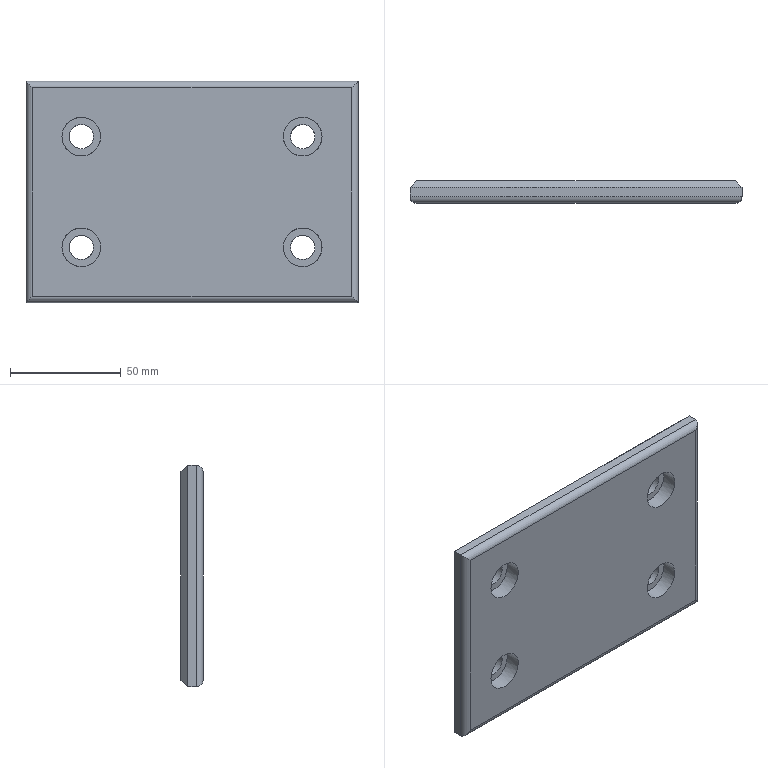Part | NX | features solid 2 | 1 solid | 26 faces | box 150 x 10 x 100 mm | volume 138955 mm3 | plane 14 | cylinder 12 | commonest cylinder face diameters 6 x4 11 x4 17.5 x4
STEP:
#1=CARTESIAN_POINT('',(-1335.,-548.,-360.));
#2=VERTEX_POINT('',#1);
#3=CARTESIAN_POINT('',(-1335.,-552.,-360.));
#4=VERTEX_POINT('',#3);
#5=CARTESIAN_POINT('',(-1335.,-545.,-360.));
#6=DIRECTION('',(0.,-1.,0.));
#7=VECTOR('',#6,1000.);
#8=LINE('',#5,#7);
#9=EDGE_CURVE('',#2,#4,#8,.T.);
#10=ORIENTED_EDGE('',*,*,#9,.F.);
#11=CARTESIAN_POINT('',(-1335.,-548.,-260.));
#12=VERTEX_POINT('',#11);
#13=CARTESIAN_POINT('',(-1335.,-548.,-260.));
#14=DIRECTION('',(0.,0.,1.));
#15=VECTOR('',#14,1000.);
#16=LINE('',#13,#15);
#17=EDGE_CURVE('',#2,#12,#16,.T.);
#18=ORIENTED_EDGE('',*,*,#17,.T.);
#19=CARTESIAN_POINT('',(-1335.,-552.,-260.));
#20=VERTEX_POINT('',#19);
#21=CARTESIAN_POINT('',(-1335.,-545.,-260.));
#22=DIRECTION('',(0.,-1.,0.));
#23=VECTOR('',#22,1000.);
#24=LINE('',#21,#23);
#25=EDGE_CURVE('',#12,#20,#24,.T.);
#26=ORIENTED_EDGE('',*,*,#25,.T.);
#27=CARTESIAN_POINT('',(-1335.,-552.,-360.));
#28=DIRECTION('',(0.,0.,-1.));
#29=VECTOR('',#28,1000.);
#30=LINE('',#27,#29);
#31=EDGE_CURVE('',#20,#4,#30,.T.);
#32=ORIENTED_EDGE('',*,*,#31,.T.);
#33=EDGE_LOOP('',(#10,#18,#26,#32));
#34=FACE_BOUND('',#33,.T.);
#35=CARTESIAN_POINT('',(-1335.,-545.,-260.));
#36=DIRECTION('',(-1.,0.,0.));
#37=DIRECTION('',(0.,0.,1.));
#38=AXIS2_PLACEMENT_3D('',#35,#36,#37);
#39=PLANE('',#38);
#40=ADVANCED_FACE('',(#34),#39,.F.);
#41=CARTESIAN_POINT('',(-1485.,-548.,-360.));
#42=VERTEX_POINT('',#41);
#43=CARTESIAN_POINT('',(-1485.,-552.,-360.));
#44=VERTEX_POINT('',#43);
#45=CARTESIAN_POINT('',(-1485.,-545.,-360.));
#46=DIRECTION('',(0.,-1.,0.));
#47=VECTOR('',#46,1000.);
#48=LINE('',#45,#47);
#49=EDGE_CURVE('',#42,#44,#48,.T.);
#50=ORIENTED_EDGE('',*,*,#49,.F.);
#51=CARTESIAN_POINT('',(-1385.,-548.,-360.));
#52=DIRECTION('',(1.,0.,0.));
#53=VECTOR('',#52,1000.);
#54=LINE('',#51,#53);
#55=EDGE_CURVE('',#42,#2,#54,.T.);
#56=ORIENTED_EDGE('',*,*,#55,.T.);
#57=ORIENTED_EDGE('',*,*,#9,.T.);
#58=CARTESIAN_POINT('',(-1485.,-552.,-360.));
#59=DIRECTION('',(-1.,0.,0.));
#60=VECTOR('',#59,1000.);
#61=LINE('',#58,#60);
#62=EDGE_CURVE('',#4,#44,#61,.T.);
#63=ORIENTED_EDGE('',*,*,#62,.T.);
#64=EDGE_LOOP('',(#50,#56,#57,#63));
#65=FACE_BOUND('',#64,.T.);
#66=CARTESIAN_POINT('',(-1385.,-545.,-360.));
#67=DIRECTION('',(0.,0.,1.));
#68=DIRECTION('',(0.,1.,0.));
#69=AXIS2_PLACEMENT_3D('',#66,#67,#68);
#70=PLANE('',#69);
#71=ADVANCED_FACE('',(#65),#70,.F.);
#72=CARTESIAN_POINT('',(-1485.,-548.,-260.));
#73=VERTEX_POINT('',#72);
#74=CARTESIAN_POINT('',(-1485.,-552.,-260.));
#75=VERTEX_POINT('',#74);
#76=CARTESIAN_POINT('',(-1485.,-545.,-260.));
#77=DIRECTION('',(0.,-1.,0.));
#78=VECTOR('',#77,1000.);
#79=LINE('',#76,#78);
#80=EDGE_CURVE('',#73,#75,#79,.T.);
#81=ORIENTED_EDGE('',*,*,#80,.F.);
#82=CARTESIAN_POINT('',(-1485.,-548.,-360.));
#83=DIRECTION('',(0.,0.,-1.));
#84=VECTOR('',#83,1000.);
#85=LINE('',#82,#84);
#86=EDGE_CURVE('',#73,#42,#85,.T.);
#87=ORIENTED_EDGE('',*,*,#86,.T.);
#88=ORIENTED_EDGE('',*,*,#49,.T.);
#89=CARTESIAN_POINT('',(-1485.,-552.,-260.));
#90=DIRECTION('',(0.,0.,1.));
#91=VECTOR('',#90,1000.);
#92=LINE('',#89,#91);
#93=EDGE_CURVE('',#44,#75,#92,.T.);
#94=ORIENTED_EDGE('',*,*,#93,.T.);
#95=EDGE_LOOP('',(#81,#87,#88,#94));
#96=FACE_BOUND('',#95,.T.);
#97=CARTESIAN_POINT('',(-1485.,-545.,-360.));
#98=DIRECTION('',(1.,0.,0.));
#99=DIRECTION('',(0.,1.,0.));
#100=AXIS2_PLACEMENT_3D('',#97,#98,#99);
#101=PLANE('',#100);
#102=ADVANCED_FACE('',(#96),#101,.F.);
#103=ORIENTED_EDGE('',*,*,#25,.F.);
#104=CARTESIAN_POINT('',(-1485.,-548.,-260.));
#105=DIRECTION('',(-1.,0.,0.));
#106=VECTOR('',#105,1000.);
#107=LINE('',#104,#106);
#108=EDGE_CURVE('',#12,#73,#107,.T.);
#109=ORIENTED_EDGE('',*,*,#108,.T.);
#110=ORIENTED_EDGE('',*,*,#80,.T.);
#111=CARTESIAN_POINT('',(-1385.,-552.,-260.));
#112=DIRECTION('',(1.,0.,0.));
#113=VECTOR('',#112,1000.);
#114=LINE('',#111,#113);
#115=EDGE_CURVE('',#75,#20,#114,.T.);
#116=ORIENTED_EDGE('',*,*,#115,.T.);
#117=EDGE_LOOP('',(#103,#109,#110,#116));
#118=FACE_BOUND('',#117,.T.);
#119=CARTESIAN_POINT('',(-1485.,-545.,-260.));
#120=DIRECTION('',(0.,0.,-1.));
#121=DIRECTION('',(-1.,0.,0.));
#122=AXIS2_PLACEMENT_3D('',#119,#120,#121);
#123=PLANE('',#122);
#124=ADVANCED_FACE('',(#118),#123,.F.);
#125=CARTESIAN_POINT('',(-1338.,-545.,-357.));
#126=VERTEX_POINT('',#125);
#127=CARTESIAN_POINT('',(-1482.,-545.,-357.));
#128=VERTEX_POINT('',#127);
#129=CARTESIAN_POINT('',(-1385.,-545.,-357.));
#130=DIRECTION('',(-1.,0.,0.));
#131=VECTOR('',#130,1000.);
#132=LINE('',#129,#131);
#133=EDGE_CURVE('',#126,#128,#132,.T.);
#134=ORIENTED_EDGE('',*,*,#133,.T.);
#135=CARTESIAN_POINT('',(-1482.,-545.,-263.));
#136=VERTEX_POINT('',#135);
#137=CARTESIAN_POINT('',(-1482.,-545.,-260.));
#138=DIRECTION('',(0.,0.,1.));
#139=VECTOR('',#138,1000.);
#140=LINE('',#137,#139);
#141=EDGE_CURVE('',#128,#136,#140,.T.);
#142=ORIENTED_EDGE('',*,*,#141,.T.);
#143=CARTESIAN_POINT('',(-1338.,-545.,-263.));
#144=VERTEX_POINT('',#143);
#145=CARTESIAN_POINT('',(-1385.,-545.,-263.));
#146=DIRECTION('',(1.,0.,0.));
#147=VECTOR('',#146,1000.);
#148=LINE('',#145,#147);
#149=EDGE_CURVE('',#136,#144,#148,.T.);
#150=ORIENTED_EDGE('',*,*,#149,.T.);
#151=CARTESIAN_POINT('',(-1338.,-545.,-260.));
#152=DIRECTION('',(0.,0.,-1.));
#153=VECTOR('',#152,1000.);
#154=LINE('',#151,#153);
#155=EDGE_CURVE('',#144,#126,#154,.T.);
#156=ORIENTED_EDGE('',*,*,#155,.T.);
#157=EDGE_LOOP('',(#134,#142,#150,#156));
#158=FACE_BOUND('',#157,.T.);
#159=CARTESIAN_POINT('',(-1454.5,-545.,-335.));
#160=VERTEX_POINT('',#159);
#161=CARTESIAN_POINT('',(-1460.,-545.,-335.));
#162=DIRECTION('',(0.,-1.,0.));
#163=DIRECTION('',(1.,0.,0.));
#164=AXIS2_PLACEMENT_3D('',#161,#162,#163);
#165=CIRCLE('',#164,5.5);
#166=EDGE_CURVE('',#160,#160,#165,.T.);
#167=ORIENTED_EDGE('',*,*,#166,.T.);
#168=EDGE_LOOP('',(#167));
#169=FACE_BOUND('',#168,.T.);
#170=CARTESIAN_POINT('',(-1454.5,-545.,-285.));
#171=VERTEX_POINT('',#170);
#172=CARTESIAN_POINT('',(-1460.,-545.,-285.));
#173=DIRECTION('',(0.,-1.,0.));
#174=DIRECTION('',(1.,0.,0.));
#175=AXIS2_PLACEMENT_3D('',#172,#173,#174);
#176=CIRCLE('',#175,5.5);
#177=EDGE_CURVE('',#171,#171,#176,.T.);
#178=ORIENTED_EDGE('',*,*,#177,.T.);
#179=EDGE_LOOP('',(#178));
#180=FACE_BOUND('',#179,.T.);
#181=CARTESIAN_POINT('',(-1354.5,-545.,-335.));
#182=VERTEX_POINT('',#181);
#183=CARTESIAN_POINT('',(-1360.,-545.,-335.));
#184=DIRECTION('',(0.,-1.,0.));
#185=DIRECTION('',(1.,0.,0.));
#186=AXIS2_PLACEMENT_3D('',#183,#184,#185);
#187=CIRCLE('',#186,5.5);
#188=EDGE_CURVE('',#182,#182,#187,.T.);
#189=ORIENTED_EDGE('',*,*,#188,.T.);
#190=EDGE_LOOP('',(#189));
#191=FACE_BOUND('',#190,.T.);
#192=CARTESIAN_POINT('',(-1354.5,-545.,-285.));
#193=VERTEX_POINT('',#192);
#194=CARTESIAN_POINT('',(-1360.,-545.,-285.));
#195=DIRECTION('',(0.,-1.,0.));
#196=DIRECTION('',(1.,0.,0.));
#197=AXIS2_PLACEMENT_3D('',#194,#195,#196);
#198=CIRCLE('',#197,5.5);
#199=EDGE_CURVE('',#193,#193,#198,.T.);
#200=ORIENTED_EDGE('',*,*,#199,.T.);
#201=EDGE_LOOP('',(#200));
#202=FACE_BOUND('',#201,.T.);
#203=CARTESIAN_POINT('',(-1385.,-545.,-260.));
#204=DIRECTION('',(0.,-1.,0.));
#205=DIRECTION('',(1.,0.,0.));
#206=AXIS2_PLACEMENT_3D('',#203,#204,#205);
#207=PLANE('',#206);
#208=ADVANCED_FACE('',(#158,#169,#180,#191,#202),#207,.F.);
#209=CARTESIAN_POINT('',(-1338.,-555.,-357.));
#210=VERTEX_POINT('',#209);
#211=CARTESIAN_POINT('',(-1338.,-555.,-263.));
#212=VERTEX_POINT('',#211);
#213=CARTESIAN_POINT('',(-1338.,-555.,-260.));
#214=DIRECTION('',(0.,0.,-1.));
#215=VECTOR('',#214,1000.);
#216=LINE('',#213,#215);
#217=EDGE_CURVE('',#210,#212,#216,.F.);
#218=ORIENTED_EDGE('',*,*,#217,.T.);
#219=CARTESIAN_POINT('',(-1482.,-555.,-263.));
#220=VERTEX_POINT('',#219);
#221=CARTESIAN_POINT('',(-1485.,-555.,-263.));
#222=DIRECTION('',(1.,0.,0.));
#223=VECTOR('',#222,1000.);
#224=LINE('',#221,#223);
#225=EDGE_CURVE('',#212,#220,#224,.F.);
#226=ORIENTED_EDGE('',*,*,#225,.T.);
#227=CARTESIAN_POINT('',(-1482.,-555.,-357.));
#228=VERTEX_POINT('',#227);
#229=CARTESIAN_POINT('',(-1482.,-555.,-360.));
#230=DIRECTION('',(0.,0.,1.));
#231=VECTOR('',#230,1000.);
#232=LINE('',#229,#231);
#233=EDGE_CURVE('',#220,#228,#232,.F.);
#234=ORIENTED_EDGE('',*,*,#233,.T.);
#235=CARTESIAN_POINT('',(-1385.,-555.,-357.));
#236=DIRECTION('',(-1.,0.,0.));
#237=VECTOR('',#236,1000.);
#238=LINE('',#235,#237);
#239=EDGE_CURVE('',#228,#210,#238,.F.);
#240=ORIENTED_EDGE('',*,*,#239,.T.);
#241=EDGE_LOOP('',(#218,#226,#234,#240));
#242=FACE_BOUND('',#241,.T.);
#243=CARTESIAN_POINT('',(-1468.75,-555.,-335.));
#244=VERTEX_POINT('',#243);
#245=CARTESIAN_POINT('',(-1460.,-555.,-335.));
#246=DIRECTION('',(0.,1.,0.));
#247=DIRECTION('',(-1.,0.,0.));
#248=AXIS2_PLACEMENT_3D('',#245,#246,#247);
#249=CIRCLE('',#248,8.75);
#250=EDGE_CURVE('',#244,#244,#249,.T.);
#251=ORIENTED_EDGE('',*,*,#250,.T.);
#252=EDGE_LOOP('',(#251));
#253=FACE_BOUND('',#252,.T.);
#254=CARTESIAN_POINT('',(-1468.75,-555.,-285.));
#255=VERTEX_POINT('',#254);
#256=CARTESIAN_POINT('',(-1460.,-555.,-285.));
#257=DIRECTION('',(0.,1.,0.));
#258=DIRECTION('',(-1.,0.,0.));
#259=AXIS2_PLACEMENT_3D('',#256,#257,#258);
#260=CIRCLE('',#259,8.75);
#261=EDGE_CURVE('',#255,#255,#260,.T.);
#262=ORIENTED_EDGE('',*,*,#261,.T.);
#263=EDGE_LOOP('',(#262));
#264=FACE_BOUND('',#263,.T.);
#265=CARTESIAN_POINT('',(-1368.75,-555.,-335.));
#266=VERTEX_POINT('',#265);
#267=CARTESIAN_POINT('',(-1360.,-555.,-335.));
#268=DIRECTION('',(0.,1.,0.));
#269=DIRECTION('',(-1.,0.,0.));
#270=AXIS2_PLACEMENT_3D('',#267,#268,#269);
#271=CIRCLE('',#270,8.75);
#272=EDGE_CURVE('',#266,#266,#271,.T.);
#273=ORIENTED_EDGE('',*,*,#272,.T.);
#274=EDGE_LOOP('',(#273));
#275=FACE_BOUND('',#274,.T.);
#276=CARTESIAN_POINT('',(-1368.75,-555.,-285.));
#277=VERTEX_POINT('',#276);
#278=CARTESIAN_POINT('',(-1360.,-555.,-285.));
#279=DIRECTION('',(0.,1.,0.));
#280=DIRECTION('',(-1.,0.,0.));
#281=AXIS2_PLACEMENT_3D('',#278,#279,#280);
#282=CIRCLE('',#281,8.75);
#283=EDGE_CURVE('',#277,#277,#282,.T.);
#284=ORIENTED_EDGE('',*,*,#283,.T.);
#285=EDGE_LOOP('',(#284));
#286=FACE_BOUND('',#285,.T.);
#287=CARTESIAN_POINT('',(-1385.,-555.,-260.));
#288=DIRECTION('',(0.,-1.,0.));
#289=DIRECTION('',(1.,0.,0.));
#290=AXIS2_PLACEMENT_3D('',#287,#288,#289);
#291=PLANE('',#290);
#292=ADVANCED_FACE('',(#242,#253,#264,#275,#286),#291,.T.);
#293=CARTESIAN_POINT('',(-1360.,-548.,-290.5));
#294=VERTEX_POINT('',#293);
#295=CARTESIAN_POINT('',(-1360.,-548.,-285.));
#296=DIRECTION('',(0.,1.,0.));
#297=DIRECTION('',(0.,0.,-1.));
#298=AXIS2_PLACEMENT_3D('',#295,#296,#297);
#299=CIRCLE('',#298,5.5);
#300=EDGE_CURVE('',#294,#294,#299,.T.);
#301=ORIENTED_EDGE('',*,*,#300,.F.);
#302=EDGE_LOOP('',(#301));
#303=FACE_BOUND('',#302,.T.);
#304=ORIENTED_EDGE('',*,*,#199,.F.);
#305=EDGE_LOOP('',(#304));
#306=FACE_BOUND('',#305,.T.);
#307=CARTESIAN_POINT('',(-1360.,-515.,-285.));
#308=DIRECTION('',(0.,1.,0.));
#309=DIRECTION('',(-1.,0.,0.));
#310=AXIS2_PLACEMENT_3D('',#307,#308,#309);
#311=CYLINDRICAL_SURFACE('',#310,5.5);
#312=ADVANCED_FACE('',(#303,#306),#311,.F.);
#313=ORIENTED_EDGE('',*,*,#300,.T.);
#314=EDGE_LOOP('',(#313));
#315=FACE_BOUND('',#314,.T.);
#316=CARTESIAN_POINT('',(-1360.,-548.,-293.75));
#317=VERTEX_POINT('',#316);
#318=CARTESIAN_POINT('',(-1360.,-548.,-285.));
#319=DIRECTION('',(0.,1.,0.));
#320=DIRECTION('',(0.,0.,-1.));
#321=AXIS2_PLACEMENT_3D('',#318,#319,#320);
#322=CIRCLE('',#321,8.75);
#323=EDGE_CURVE('',#317,#317,#322,.T.);
#324=ORIENTED_EDGE('',*,*,#323,.F.);
#325=EDGE_LOOP('',(#324));
#326=FACE_BOUND('',#325,.T.);
#327=CARTESIAN_POINT('',(-1360.,-548.,-285.));
#328=DIRECTION('',(0.,1.,0.));
#329=DIRECTION('',(-1.,0.,0.));
#330=AXIS2_PLACEMENT_3D('',#327,#328,#329);
#331=PLANE('',#330);
#332=ADVANCED_FACE('',(#315,#326),#331,.F.);
#333=ORIENTED_EDGE('',*,*,#323,.T.);
#334=EDGE_LOOP('',(#333));
#335=FACE_BOUND('',#334,.T.);
#336=ORIENTED_EDGE('',*,*,#283,.F.);
#337=EDGE_LOOP('',(#336));
#338=FACE_BOUND('',#337,.T.);
#339=CARTESIAN_POINT('',(-1360.,-565.,-285.));
#340=DIRECTION('',(0.,1.,0.));
#341=DIRECTION('',(-1.,0.,0.));
#342=AXIS2_PLACEMENT_3D('',#339,#340,#341);
#343=CYLINDRICAL_SURFACE('',#342,8.75);
#344=ADVANCED_FACE('',(#335,#338),#343,.F.);
#345=CARTESIAN_POINT('',(-1360.,-548.,-340.5));
#346=VERTEX_POINT('',#345);
#347=CARTESIAN_POINT('',(-1360.,-548.,-335.));
#348=DIRECTION('',(0.,1.,0.));
#349=DIRECTION('',(0.,0.,-1.));
#350=AXIS2_PLACEMENT_3D('',#347,#348,#349);
#351=CIRCLE('',#350,5.5);
#352=EDGE_CURVE('',#346,#346,#351,.T.);
#353=ORIENTED_EDGE('',*,*,#352,.F.);
#354=EDGE_LOOP('',(#353));
#355=FACE_BOUND('',#354,.T.);
#356=ORIENTED_EDGE('',*,*,#188,.F.);
#357=EDGE_LOOP('',(#356));
#358=FACE_BOUND('',#357,.T.);
#359=CARTESIAN_POINT('',(-1360.,-515.,-335.));
#360=DIRECTION('',(0.,1.,0.));
#361=DIRECTION('',(-1.,0.,0.));
#362=AXIS2_PLACEMENT_3D('',#359,#360,#361);
#363=CYLINDRICAL_SURFACE('',#362,5.5);
#364=ADVANCED_FACE('',(#355,#358),#363,.F.);
#365=ORIENTED_EDGE('',*,*,#352,.T.);
#366=EDGE_LOOP('',(#365));
#367=FACE_BOUND('',#366,.T.);
#368=CARTESIAN_POINT('',(-1360.,-548.,-343.75));
#369=VERTEX_POINT('',#368);
#370=CARTESIAN_POINT('',(-1360.,-548.,-335.));
#371=DIRECTION('',(0.,1.,0.));
#372=DIRECTION('',(0.,0.,-1.));
#373=AXIS2_PLACEMENT_3D('',#370,#371,#372);
#374=CIRCLE('',#373,8.75);
#375=EDGE_CURVE('',#369,#369,#374,.T.);
#376=ORIENTED_EDGE('',*,*,#375,.F.);
#377=EDGE_LOOP('',(#376));
#378=FACE_BOUND('',#377,.T.);
#379=CARTESIAN_POINT('',(-1360.,-548.,-335.));
#380=DIRECTION('',(0.,1.,0.));
#381=DIRECTION('',(-1.,0.,0.));
#382=AXIS2_PLACEMENT_3D('',#379,#380,#381);
#383=PLANE('',#382);
#384=ADVANCED_FACE('',(#367,#378),#383,.F.);
#385=ORIENTED_EDGE('',*,*,#375,.T.);
#386=EDGE_LOOP('',(#385));
#387=FACE_BOUND('',#386,.T.);
#388=ORIENTED_EDGE('',*,*,#272,.F.);
#389=EDGE_LOOP('',(#388));
#390=FACE_BOUND('',#389,.T.);
#391=CARTESIAN_POINT('',(-1360.,-565.,-335.));
#392=DIRECTION('',(0.,1.,0.));
#393=DIRECTION('',(-1.,0.,0.));
#394=AXIS2_PLACEMENT_3D('',#391,#392,#393);
#395=CYLINDRICAL_SURFACE('',#394,8.75);
#396=ADVANCED_FACE('',(#387,#390),#395,.F.);
#397=CARTESIAN_POINT('',(-1460.,-548.,-290.5));
#398=VERTEX_POINT('',#397);
#399=CARTESIAN_POINT('',(-1460.,-548.,-285.));
#400=DIRECTION('',(0.,1.,0.));
#401=DIRECTION('',(0.,0.,-1.));
#402=AXIS2_PLACEMENT_3D('',#399,#400,#401);
#403=CIRCLE('',#402,5.5);
#404=EDGE_CURVE('',#398,#398,#403,.T.);
#405=ORIENTED_EDGE('',*,*,#404,.F.);
#406=EDGE_LOOP('',(#405));
#407=FACE_BOUND('',#406,.T.);
#408=ORIENTED_EDGE('',*,*,#177,.F.);
#409=EDGE_LOOP('',(#408));
#410=FACE_BOUND('',#409,.T.);
#411=CARTESIAN_POINT('',(-1460.,-515.,-285.));
#412=DIRECTION('',(0.,1.,0.));
#413=DIRECTION('',(-1.,0.,0.));
#414=AXIS2_PLACEMENT_3D('',#411,#412,#413);
#415=CYLINDRICAL_SURFACE('',#414,5.5);
#416=ADVANCED_FACE('',(#407,#410),#415,.F.);
#417=ORIENTED_EDGE('',*,*,#404,.T.);
#418=EDGE_LOOP('',(#417));
#419=FACE_BOUND('',#418,.T.);
#420=CARTESIAN_POINT('',(-1460.,-548.,-293.75));
#421=VERTEX_POINT('',#420);
#422=CARTESIAN_POINT('',(-1460.,-548.,-285.));
#423=DIRECTION('',(0.,1.,0.));
#424=DIRECTION('',(0.,0.,-1.));
#425=AXIS2_PLACEMENT_3D('',#422,#423,#424);
#426=CIRCLE('',#425,8.75);
#427=EDGE_CURVE('',#421,#421,#426,.T.);
#428=ORIENTED_EDGE('',*,*,#427,.F.);
#429=EDGE_LOOP('',(#428));
#430=FACE_BOUND('',#429,.T.);
#431=CARTESIAN_POINT('',(-1460.,-548.,-285.));
#432=DIRECTION('',(0.,1.,0.));
#433=DIRECTION('',(-1.,0.,0.));
#434=AXIS2_PLACEMENT_3D('',#431,#432,#433);
#435=PLANE('',#434);
#436=ADVANCED_FACE('',(#419,#430),#435,.F.);
#437=ORIENTED_EDGE('',*,*,#427,.T.);
#438=EDGE_LOOP('',(#437));
#439=FACE_BOUND('',#438,.T.);
#440=ORIENTED_EDGE('',*,*,#261,.F.);
#441=EDGE_LOOP('',(#440));
#442=FACE_BOUND('',#441,.T.);
#443=CARTESIAN_POINT('',(-1460.,-565.,-285.));
#444=DIRECTION('',(0.,1.,0.));
#445=DIRECTION('',(-1.,0.,0.));
#446=AXIS2_PLACEMENT_3D('',#443,#444,#445);
#447=CYLINDRICAL_SURFACE('',#446,8.75);
#448=ADVANCED_FACE('',(#439,#442),#447,.F.);
#449=CARTESIAN_POINT('',(-1460.,-548.,-340.5));
#450=VERTEX_POINT('',#449);
#451=CARTESIAN_POINT('',(-1460.,-548.,-335.));
#452=DIRECTION('',(0.,1.,0.));
#453=DIRECTION('',(0.,0.,-1.));
#454=AXIS2_PLACEMENT_3D('',#451,#452,#453);
#455=CIRCLE('',#454,5.5);
#456=EDGE_CURVE('',#450,#450,#455,.T.);
#457=ORIENTED_EDGE('',*,*,#456,.F.);
#458=EDGE_LOOP('',(#457));
#459=FACE_BOUND('',#458,.T.);
#460=ORIENTED_EDGE('',*,*,#166,.F.);
#461=EDGE_LOOP('',(#460));
#462=FACE_BOUND('',#461,.T.);
#463=CARTESIAN_POINT('',(-1460.,-515.,-335.));
#464=DIRECTION('',(0.,1.,0.));
#465=DIRECTION('',(-1.,0.,0.));
#466=AXIS2_PLACEMENT_3D('',#463,#464,#465);
#467=CYLINDRICAL_SURFACE('',#466,5.5);
#468=ADVANCED_FACE('',(#459,#462),#467,.F.);
#469=ORIENTED_EDGE('',*,*,#456,.T.);
#470=EDGE_LOOP('',(#469));
#471=FACE_BOUND('',#470,.T.);
#472=CARTESIAN_POINT('',(-1460.,-548.,-343.75));
#473=VERTEX_POINT('',#472);
#474=CARTESIAN_POINT('',(-1460.,-548.,-335.));
#475=DIRECTION('',(0.,1.,0.));
#476=DIRECTION('',(0.,0.,-1.));
#477=AXIS2_PLACEMENT_3D('',#474,#475,#476);
#478=CIRCLE('',#477,8.75);
#479=EDGE_CURVE('',#473,#473,#478,.T.);
#480=ORIENTED_EDGE('',*,*,#479,.F.);
#481=EDGE_LOOP('',(#480));
#482=FACE_BOUND('',#481,.T.);
#483=CARTESIAN_POINT('',(-1460.,-548.,-335.));
#484=DIRECTION('',(0.,1.,0.));
#485=DIRECTION('',(-1.,0.,0.));
#486=AXIS2_PLACEMENT_3D('',#483,#484,#485);
#487=PLANE('',#486);
#488=ADVANCED_FACE('',(#471,#482),#487,.F.);
#489=ORIENTED_EDGE('',*,*,#479,.T.);
#490=EDGE_LOOP('',(#489));
#491=FACE_BOUND('',#490,.T.);
#492=ORIENTED_EDGE('',*,*,#250,.F.);
#493=EDGE_LOOP('',(#492));
#494=FACE_BOUND('',#493,.T.);
#495=CARTESIAN_POINT('',(-1460.,-565.,-335.));
#496=DIRECTION('',(0.,1.,0.));
#497=DIRECTION('',(-1.,0.,0.));
#498=AXIS2_PLACEMENT_3D('',#495,#496,#497);
#499=CYLINDRICAL_SURFACE('',#498,8.75);
#500=ADVANCED_FACE('',(#491,#494),#499,.F.);
#501=CARTESIAN_POINT('',(-1338.,-552.,-357.));
#502=DIRECTION('',(0.7071,0.,0.7071));
#503=DIRECTION('',(-0.7071,0.,0.7071));
#504=AXIS2_PLACEMENT_3D('',#501,#502,#503);
#505=ELLIPSE('',#504,4.243,3.);
#506=EDGE_CURVE('',#210,#4,#505,.T.);
#507=ORIENTED_EDGE('',*,*,#506,.F.);
#508=ORIENTED_EDGE('',*,*,#239,.F.);
#509=CARTESIAN_POINT('',(-1482.,-552.,-357.));
#510=DIRECTION('',(0.7071,0.,-0.7071));
#511=DIRECTION('',(0.7071,0.,0.7071));
#512=AXIS2_PLACEMENT_3D('',#509,#510,#511);
#513=ELLIPSE('',#512,4.243,3.);
#514=EDGE_CURVE('',#44,#228,#513,.F.);
#515=ORIENTED_EDGE('',*,*,#514,.F.);
#516=ORIENTED_EDGE('',*,*,#62,.F.);
#517=EDGE_LOOP('',(#507,#508,#515,#516));
#518=FACE_BOUND('',#517,.T.);
#519=CARTESIAN_POINT('',(-1385.,-552.,-357.));
#520=DIRECTION('',(1.,0.,0.));
#521=DIRECTION('',(0.,1.,0.));
#522=AXIS2_PLACEMENT_3D('',#519,#520,#521);
#523=CYLINDRICAL_SURFACE('',#522,3.);
#524=ADVANCED_FACE('',(#518),#523,.T.);
#525=ORIENTED_EDGE('',*,*,#514,.T.);
#526=ORIENTED_EDGE('',*,*,#233,.F.);
#527=CARTESIAN_POINT('',(-1482.,-552.,-263.));
#528=DIRECTION('',(-0.7071,0.,-0.7071));
#529=DIRECTION('',(0.7071,0.,-0.7071));
#530=AXIS2_PLACEMENT_3D('',#527,#528,#529);
#531=ELLIPSE('',#530,4.243,3.);
#532=EDGE_CURVE('',#75,#220,#531,.F.);
#533=ORIENTED_EDGE('',*,*,#532,.F.);
#534=ORIENTED_EDGE('',*,*,#93,.F.);
#535=EDGE_LOOP('',(#525,#526,#533,#534));
#536=FACE_BOUND('',#535,.T.);
#537=CARTESIAN_POINT('',(-1482.,-552.,-360.));
#538=DIRECTION('',(0.,0.,-1.));
#539=DIRECTION('',(0.,-1.,0.));
#540=AXIS2_PLACEMENT_3D('',#537,#538,#539);
#541=CYLINDRICAL_SURFACE('',#540,3.);
#542=ADVANCED_FACE('',(#536),#541,.T.);
#543=ORIENTED_EDGE('',*,*,#506,.T.);
#544=ORIENTED_EDGE('',*,*,#31,.F.);
#545=CARTESIAN_POINT('',(-1338.,-552.,-263.));
#546=DIRECTION('',(-0.7071,0.,0.7071));
#547=DIRECTION('',(0.7071,0.,0.7071));
#548=AXIS2_PLACEMENT_3D('',#545,#546,#547);
#549=ELLIPSE('',#548,4.243,3.);
#550=EDGE_CURVE('',#212,#20,#549,.T.);
#551=ORIENTED_EDGE('',*,*,#550,.F.);
#552=ORIENTED_EDGE('',*,*,#217,.F.);
#553=EDGE_LOOP('',(#543,#544,#551,#552));
#554=FACE_BOUND('',#553,.T.);
#555=CARTESIAN_POINT('',(-1338.,-552.,-260.));
#556=DIRECTION('',(0.,0.,1.));
#557=DIRECTION('',(1.,0.,0.));
#558=AXIS2_PLACEMENT_3D('',#555,#556,#557);
#559=CYLINDRICAL_SURFACE('',#558,3.);
#560=ADVANCED_FACE('',(#554),#559,.T.);
#561=ORIENTED_EDGE('',*,*,#532,.T.);
#562=ORIENTED_EDGE('',*,*,#225,.F.);
#563=ORIENTED_EDGE('',*,*,#550,.T.);
#564=ORIENTED_EDGE('',*,*,#115,.F.);
#565=EDGE_LOOP('',(#561,#562,#563,#564));
#566=FACE_BOUND('',#565,.T.);
#567=CARTESIAN_POINT('',(-1485.,-552.,-263.));
#568=DIRECTION('',(-1.,0.,0.));
#569=DIRECTION('',(0.,0.,1.));
#570=AXIS2_PLACEMENT_3D('',#567,#568,#569);
#571=CYLINDRICAL_SURFACE('',#570,3.);
#572=ADVANCED_FACE('',(#566),#571,.T.);
#573=CARTESIAN_POINT('',(-1337.,-546.,-262.));
#574=DIRECTION('',(-0.5774,0.5774,-0.5774));
#575=VECTOR('',#574,1000.);
#576=LINE('',#573,#575);
#577=EDGE_CURVE('',#12,#144,#576,.T.);
#578=ORIENTED_EDGE('',*,*,#577,.F.);
#579=ORIENTED_EDGE('',*,*,#17,.F.);
#580=CARTESIAN_POINT('',(-1370.333,-512.667,-324.667));
#581=DIRECTION('',(-0.5774,0.5774,0.5774));
#582=VECTOR('',#581,1000.);
#583=LINE('',#580,#582);
#584=EDGE_CURVE('',#126,#2,#583,.F.);
#585=ORIENTED_EDGE('',*,*,#584,.F.);
#586=ORIENTED_EDGE('',*,*,#155,.F.);
#587=EDGE_LOOP('',(#578,#579,#585,#586));
#588=FACE_BOUND('',#587,.T.);
#589=CARTESIAN_POINT('',(-1338.,-545.,-260.));
#590=DIRECTION('',(-0.7071,-0.7071,0.));
#591=DIRECTION('',(0.7071,-0.7071,0.));
#592=AXIS2_PLACEMENT_3D('',#589,#590,#591);
#593=PLANE('',#592);
#594=ADVANCED_FACE('',(#588),#593,.F.);
#595=ORIENTED_EDGE('',*,*,#584,.T.);
#596=ORIENTED_EDGE('',*,*,#55,.F.);
#597=CARTESIAN_POINT('',(-1449.667,-512.667,-324.667));
#598=DIRECTION('',(0.5774,0.5774,0.5774));
#599=VECTOR('',#598,1000.);
#600=LINE('',#597,#599);
#601=EDGE_CURVE('',#128,#42,#600,.F.);
#602=ORIENTED_EDGE('',*,*,#601,.F.);
#603=ORIENTED_EDGE('',*,*,#133,.F.);
#604=EDGE_LOOP('',(#595,#596,#602,#603));
#605=FACE_BOUND('',#604,.T.);
#606=CARTESIAN_POINT('',(-1385.,-545.,-357.));
#607=DIRECTION('',(0.,-0.7071,0.7071));
#608=DIRECTION('',(0.,0.7071,0.7071));
#609=AXIS2_PLACEMENT_3D('',#606,#607,#608);
#610=PLANE('',#609);
#611=ADVANCED_FACE('',(#605),#610,.F.);
#612=ORIENTED_EDGE('',*,*,#577,.T.);
#613=ORIENTED_EDGE('',*,*,#149,.F.);
#614=CARTESIAN_POINT('',(-1449.667,-512.667,-295.333));
#615=DIRECTION('',(-0.5774,-0.5774,0.5774));
#616=VECTOR('',#615,1000.);
#617=LINE('',#614,#616);
#618=EDGE_CURVE('',#73,#136,#617,.F.);
#619=ORIENTED_EDGE('',*,*,#618,.F.);
#620=ORIENTED_EDGE('',*,*,#108,.F.);
#621=EDGE_LOOP('',(#612,#613,#619,#620));
#622=FACE_BOUND('',#621,.T.);
#623=CARTESIAN_POINT('',(-1385.,-545.,-263.));
#624=DIRECTION('',(0.,-0.7071,-0.7071));
#625=DIRECTION('',(0.,-0.7071,0.7071));
#626=AXIS2_PLACEMENT_3D('',#623,#624,#625);
#627=PLANE('',#626);
#628=ADVANCED_FACE('',(#622),#627,.F.);
#629=ORIENTED_EDGE('',*,*,#601,.T.);
#630=ORIENTED_EDGE('',*,*,#86,.F.);
#631=ORIENTED_EDGE('',*,*,#618,.T.);
#632=ORIENTED_EDGE('',*,*,#141,.F.);
#633=EDGE_LOOP('',(#629,#630,#631,#632));
#634=FACE_BOUND('',#633,.T.);
#635=CARTESIAN_POINT('',(-1482.,-545.,-260.));
#636=DIRECTION('',(0.7071,-0.7071,0.));
#637=DIRECTION('',(0.7071,0.7071,0.));
#638=AXIS2_PLACEMENT_3D('',#635,#636,#637);
#639=PLANE('',#638);
#640=ADVANCED_FACE('',(#634),#639,.F.);
#641=CLOSED_SHELL('',(#40,#71,#102,#124,#208,#292,#312,#332,#344,#364,#384,#396,#416,#436,#448,#468,#488,#500,#524,#542,#560,#572,#594,#611,#628,#640));
#642=MANIFOLD_SOLID_BREP('',#641);
#643=(LENGTH_UNIT()NAMED_UNIT(*)SI_UNIT(.MILLI.,.METRE.));
#644=UNCERTAINTY_MEASURE_WITH_UNIT(LENGTH_MEASURE(0.00001),#643,'','');
#645=(NAMED_UNIT(*)PLANE_ANGLE_UNIT()SI_UNIT($,.RADIAN.));
#646=(NAMED_UNIT(*)SI_UNIT($,.STERADIAN.)SOLID_ANGLE_UNIT());
#647=(GEOMETRIC_REPRESENTATION_CONTEXT(3)GLOBAL_UNCERTAINTY_ASSIGNED_CONTEXT((#644))GLOBAL_UNIT_ASSIGNED_CONTEXT((#643,#645,#646))REPRESENTATION_CONTEXT('',''));
#648=ADVANCED_BREP_SHAPE_REPRESENTATION('',(#642),#647);